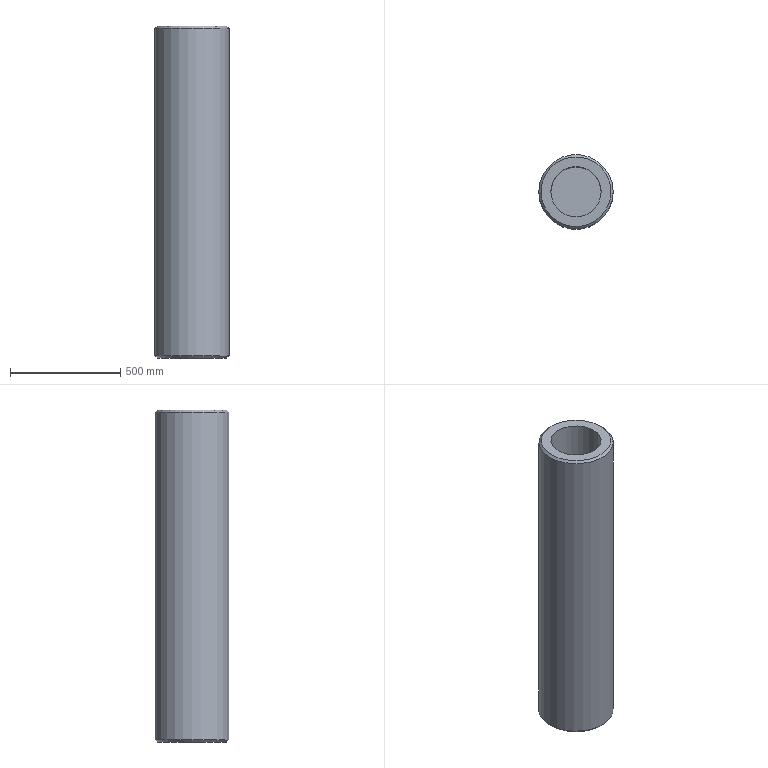Part | NX | features 立柱缸二级 2 | 1 solid | 7 faces | box 337.48 x 337.48 x 1508 mm | volume 82514797 mm3 | plane 3 | cylinder 2 | cone 2 | commonest cylinder face diameters 228.3 x1 337.48 x1
STEP:
#1=CARTESIAN_POINT('',(168.74,0.,10.));
#2=VERTEX_POINT('',#1);
#3=CARTESIAN_POINT('',(0.,0.,10.));
#4=DIRECTION('',(0.,0.,1.));
#5=DIRECTION('',(1.,0.,0.));
#6=AXIS2_PLACEMENT_3D('',#3,#4,#5);
#7=CIRCLE('',#6,168.74);
#8=EDGE_CURVE('',#2,#2,#7,.T.);
#9=ORIENTED_EDGE('',*,*,#8,.T.);
#10=EDGE_LOOP('',(#9));
#11=FACE_BOUND('',#10,.T.);
#12=CARTESIAN_POINT('',(168.74,0.,1498.224));
#13=VERTEX_POINT('',#12);
#14=CARTESIAN_POINT('',(0.,0.,1498.224));
#15=DIRECTION('',(0.,0.,1.));
#16=DIRECTION('',(1.,0.,0.));
#17=AXIS2_PLACEMENT_3D('',#14,#15,#16);
#18=CIRCLE('',#17,168.74);
#19=EDGE_CURVE('',#13,#13,#18,.F.);
#20=ORIENTED_EDGE('',*,*,#19,.T.);
#21=EDGE_LOOP('',(#20));
#22=FACE_BOUND('',#21,.T.);
#23=CARTESIAN_POINT('',(0.,0.,1508.224));
#24=DIRECTION('',(0.,0.,-1.));
#25=DIRECTION('',(-1.,0.,0.));
#26=AXIS2_PLACEMENT_3D('',#23,#24,#25);
#27=CYLINDRICAL_SURFACE('',#26,168.74);
#28=ADVANCED_FACE('',(#11,#22),#27,.T.);
#29=CARTESIAN_POINT('',(158.74,0.,1508.224));
#30=VERTEX_POINT('',#29);
#31=CARTESIAN_POINT('',(0.,0.,1508.224));
#32=DIRECTION('',(0.,0.,1.));
#33=DIRECTION('',(1.,0.,0.));
#34=AXIS2_PLACEMENT_3D('',#31,#32,#33);
#35=CIRCLE('',#34,158.74);
#36=EDGE_CURVE('',#30,#30,#35,.T.);
#37=ORIENTED_EDGE('',*,*,#36,.T.);
#38=EDGE_LOOP('',(#37));
#39=FACE_BOUND('',#38,.T.);
#40=CARTESIAN_POINT('',(114.15,0.,1508.224));
#41=VERTEX_POINT('',#40);
#42=CARTESIAN_POINT('',(0.,0.,1508.224));
#43=DIRECTION('',(0.,0.,1.));
#44=DIRECTION('',(1.,0.,0.));
#45=AXIS2_PLACEMENT_3D('',#42,#43,#44);
#46=CIRCLE('',#45,114.15);
#47=EDGE_CURVE('',#41,#41,#46,.T.);
#48=ORIENTED_EDGE('',*,*,#47,.F.);
#49=EDGE_LOOP('',(#48));
#50=FACE_BOUND('',#49,.T.);
#51=CARTESIAN_POINT('',(0.,0.,1508.224));
#52=DIRECTION('',(0.,0.,1.));
#53=DIRECTION('',(1.,0.,0.));
#54=AXIS2_PLACEMENT_3D('',#51,#52,#53);
#55=PLANE('',#54);
#56=ADVANCED_FACE('',(#39,#50),#55,.T.);
#57=CARTESIAN_POINT('',(158.74,0.,0.));
#58=VERTEX_POINT('',#57);
#59=CARTESIAN_POINT('',(0.,0.,0.));
#60=DIRECTION('',(0.,0.,1.));
#61=DIRECTION('',(1.,0.,0.));
#62=AXIS2_PLACEMENT_3D('',#59,#60,#61);
#63=CIRCLE('',#62,158.74);
#64=EDGE_CURVE('',#58,#58,#63,.F.);
#65=ORIENTED_EDGE('',*,*,#64,.T.);
#66=EDGE_LOOP('',(#65));
#67=FACE_BOUND('',#66,.T.);
#68=CARTESIAN_POINT('',(0.,0.,0.));
#69=DIRECTION('',(0.,0.,1.));
#70=DIRECTION('',(1.,0.,0.));
#71=AXIS2_PLACEMENT_3D('',#68,#69,#70);
#72=PLANE('',#71);
#73=ADVANCED_FACE('',(#67),#72,.F.);
#74=CARTESIAN_POINT('',(114.15,0.,230.764));
#75=VERTEX_POINT('',#74);
#76=CARTESIAN_POINT('',(0.,0.,230.764));
#77=DIRECTION('',(0.,0.,1.));
#78=DIRECTION('',(1.,0.,0.));
#79=AXIS2_PLACEMENT_3D('',#76,#77,#78);
#80=CIRCLE('',#79,114.15);
#81=EDGE_CURVE('',#75,#75,#80,.T.);
#82=ORIENTED_EDGE('',*,*,#81,.F.);
#83=EDGE_LOOP('',(#82));
#84=FACE_BOUND('',#83,.T.);
#85=ORIENTED_EDGE('',*,*,#47,.T.);
#86=EDGE_LOOP('',(#85));
#87=FACE_BOUND('',#86,.T.);
#88=CARTESIAN_POINT('',(0.,0.,230.764));
#89=DIRECTION('',(0.,0.,1.));
#90=DIRECTION('',(1.,0.,0.));
#91=AXIS2_PLACEMENT_3D('',#88,#89,#90);
#92=CYLINDRICAL_SURFACE('',#91,114.15);
#93=ADVANCED_FACE('',(#84,#87),#92,.F.);
#94=ORIENTED_EDGE('',*,*,#81,.T.);
#95=EDGE_LOOP('',(#94));
#96=FACE_BOUND('',#95,.T.);
#97=CARTESIAN_POINT('',(0.,0.,230.764));
#98=DIRECTION('',(0.,0.,1.));
#99=DIRECTION('',(1.,0.,0.));
#100=AXIS2_PLACEMENT_3D('',#97,#98,#99);
#101=PLANE('',#100);
#102=ADVANCED_FACE('',(#96),#101,.T.);
#103=ORIENTED_EDGE('',*,*,#19,.F.);
#104=EDGE_LOOP('',(#103));
#105=FACE_BOUND('',#104,.T.);
#106=ORIENTED_EDGE('',*,*,#36,.F.);
#107=EDGE_LOOP('',(#106));
#108=FACE_BOUND('',#107,.T.);
#109=CARTESIAN_POINT('',(0.,0.,1508.224));
#110=DIRECTION('',(0.,0.,-1.));
#111=DIRECTION('',(-1.,0.,0.));
#112=AXIS2_PLACEMENT_3D('',#109,#110,#111);
#113=CONICAL_SURFACE('',#112,158.74,0.7854);
#114=ADVANCED_FACE('',(#105,#108),#113,.T.);
#115=ORIENTED_EDGE('',*,*,#64,.F.);
#116=EDGE_LOOP('',(#115));
#117=FACE_BOUND('',#116,.T.);
#118=ORIENTED_EDGE('',*,*,#8,.F.);
#119=EDGE_LOOP('',(#118));
#120=FACE_BOUND('',#119,.T.);
#121=CARTESIAN_POINT('',(0.,0.,10.));
#122=DIRECTION('',(0.,0.,1.));
#123=DIRECTION('',(1.,0.,0.));
#124=AXIS2_PLACEMENT_3D('',#121,#122,#123);
#125=CONICAL_SURFACE('',#124,168.74,0.7854);
#126=ADVANCED_FACE('',(#117,#120),#125,.T.);
#127=CLOSED_SHELL('',(#28,#56,#73,#93,#102,#114,#126));
#128=MANIFOLD_SOLID_BREP('',#127);
#129=(LENGTH_UNIT()NAMED_UNIT(*)SI_UNIT(.MILLI.,.METRE.));
#130=UNCERTAINTY_MEASURE_WITH_UNIT(LENGTH_MEASURE(0.00001),#129,'','');
#131=(NAMED_UNIT(*)PLANE_ANGLE_UNIT()SI_UNIT($,.RADIAN.));
#132=(NAMED_UNIT(*)SI_UNIT($,.STERADIAN.)SOLID_ANGLE_UNIT());
#133=(GEOMETRIC_REPRESENTATION_CONTEXT(3)GLOBAL_UNCERTAINTY_ASSIGNED_CONTEXT((#130))GLOBAL_UNIT_ASSIGNED_CONTEXT((#129,#131,#132))REPRESENTATION_CONTEXT('',''));
#134=ADVANCED_BREP_SHAPE_REPRESENTATION('',(#128),#133);